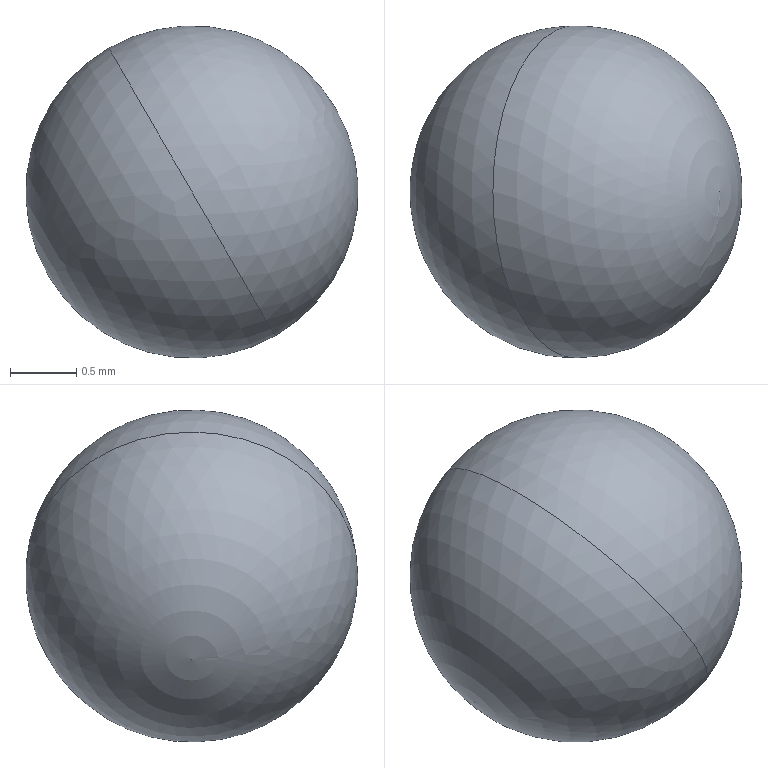Part | SolidWorks | features BaseBody 1 | 1 solid | 2 faces | box 2.5 x 2.5 x 2.5 mm | volume 8.181 mm3 | sphere 2
STEP:
#1=CARTESIAN_POINT('',(230.125,171.15,-1.083));
#2=VERTEX_POINT('',#1);
#3=CARTESIAN_POINT('',(228.875,171.15,1.083));
#4=VERTEX_POINT('',#3);
#5=CARTESIAN_POINT('',(229.5,171.15,0.));
#6=DIRECTION('',(-0.866,0.,-0.5));
#7=DIRECTION('',(-0.5,0.,0.866));
#8=AXIS2_PLACEMENT_3D('',#5,#6,#7);
#9=CIRCLE('',#8,1.25);
#10=EDGE_CURVE('',#2,#4,#9,.T.);
#11=ORIENTED_EDGE('',*,*,#10,.F.);
#12=CARTESIAN_POINT('',(229.5,171.15,0.));
#13=DIRECTION('',(0.866,0.,0.5));
#14=DIRECTION('',(0.5,0.,-0.866));
#15=AXIS2_PLACEMENT_3D('',#12,#13,#14);
#16=CIRCLE('',#15,1.25);
#17=EDGE_CURVE('',#2,#4,#16,.T.);
#18=ORIENTED_EDGE('',*,*,#17,.T.);
#19=EDGE_LOOP('',(#11,#18));
#20=FACE_OUTER_BOUND('',#19,.T.);
#21=CARTESIAN_POINT('',(229.5,171.15,0.));
#22=DIRECTION('',(0.866,0.,0.5));
#23=DIRECTION('',(0.,-1.,0.));
#24=AXIS2_PLACEMENT_3D('',#21,#22,#23);
#25=SPHERICAL_SURFACE('',#24,1.25);
#26=ADVANCED_FACE('',(#20),#25,.T.);
#27=ORIENTED_EDGE('',*,*,#17,.F.);
#28=ORIENTED_EDGE('',*,*,#10,.T.);
#29=EDGE_LOOP('',(#27,#28));
#30=FACE_OUTER_BOUND('',#29,.T.);
#31=CARTESIAN_POINT('',(229.5,171.15,0.));
#32=DIRECTION('',(0.866,0.,0.5));
#33=DIRECTION('',(0.,-1.,0.));
#34=AXIS2_PLACEMENT_3D('',#31,#32,#33);
#35=SPHERICAL_SURFACE('',#34,1.25);
#36=ADVANCED_FACE('',(#30),#35,.T.);
#37=CLOSED_SHELL('',(#26,#36));
#38=MANIFOLD_SOLID_BREP('',#37);
#39=CARTESIAN_POINT('',(0.,0.,0.));
#40=DIRECTION('',(0.,0.,1.));
#41=DIRECTION('',(1.,0.,0.));
#42=AXIS2_PLACEMENT_3D('',#39,#40,#41);
#43=(LENGTH_UNIT()NAMED_UNIT(*)SI_UNIT(.MILLI.,.METRE.));
#44=UNCERTAINTY_MEASURE_WITH_UNIT(LENGTH_MEASURE(0.00001),#43,'','');
#45=(NAMED_UNIT(*)PLANE_ANGLE_UNIT()SI_UNIT($,.RADIAN.));
#46=(NAMED_UNIT(*)SI_UNIT($,.STERADIAN.)SOLID_ANGLE_UNIT());
#47=(GEOMETRIC_REPRESENTATION_CONTEXT(3)GLOBAL_UNCERTAINTY_ASSIGNED_CONTEXT((#44))GLOBAL_UNIT_ASSIGNED_CONTEXT((#43,#45,#46))REPRESENTATION_CONTEXT('',''));
#48=ADVANCED_BREP_SHAPE_REPRESENTATION('',(#38,#42),#47);